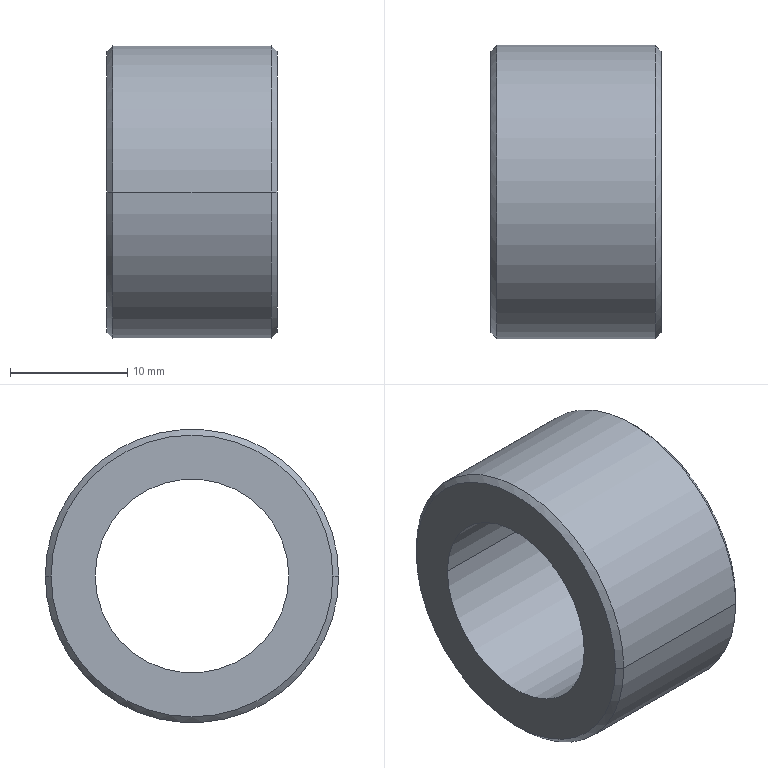Part | STEP file | J452-EBZ05-06-04 | 1 solid | 10 faces | box 14.5 x 25 x 25 mm | volume 3998 mm3 | cone 4 | cylinder 4 | plane 2 | commonest cylinder face diameters 16.5 x2 25 x2
STEP:
#1=CARTESIAN_POINT('',(0.,0.,0.));
#2=DIRECTION('',(0.,0.,1.));
#3=DIRECTION('',(1.,0.,0.));
#4=AXIS2_PLACEMENT_3D('',#1,#2,#3);
#5=CARTESIAN_POINT('',(14.5,-12.,0.));
#6=VERTEX_POINT('',#5);
#7=CARTESIAN_POINT('',(14.5,12.,0.));
#8=VERTEX_POINT('',#7);
#9=CARTESIAN_POINT('',(14.5,0.,0.));
#10=DIRECTION('',(1.,0.,0.));
#11=DIRECTION('',(0.,-1.,0.));
#12=AXIS2_PLACEMENT_3D('',#9,#10,#11);
#13=CIRCLE('',#12,12.);
#14=CARTESIAN_POINT('',(14.,0.,0.));
#15=DIRECTION('',(-1.,0.,0.));
#16=DIRECTION('',(0.,1.,0.));
#17=AXIS2_PLACEMENT_3D('',#14,#15,#16);
#18=CONICAL_SURFACE('',#17,12.5,0.7854);
#19=CARTESIAN_POINT('',(3.142,-0.5));
#20=DIRECTION('',(-1.,0.));
#21=VECTOR('',#20,1.);
#22=LINE('',#19,#21);
#23=(GEOMETRIC_REPRESENTATION_CONTEXT(2)PARAMETRIC_REPRESENTATION_CONTEXT()REPRESENTATION_CONTEXT('',''));
#24=DEFINITIONAL_REPRESENTATION('',(#22),#23);
#25=PCURVE('',#18,#24);
#26=CARTESIAN_POINT('',(14.5,0.,0.));
#27=DIRECTION('',(1.,0.,0.));
#28=DIRECTION('',(0.,-1.,0.));
#29=AXIS2_PLACEMENT_3D('',#26,#27,#28);
#30=PLANE('',#29);
#31=CARTESIAN_POINT('',(0.,0.));
#32=DIRECTION('',(1.,0.));
#33=AXIS2_PLACEMENT_2D('',#31,#32);
#34=CIRCLE('',#33,12.);
#35=(GEOMETRIC_REPRESENTATION_CONTEXT(2)PARAMETRIC_REPRESENTATION_CONTEXT()REPRESENTATION_CONTEXT('',''));
#36=DEFINITIONAL_REPRESENTATION('',(#34),#35);
#37=PCURVE('',#30,#36);
#38=SURFACE_CURVE('',#13,(#25,#37),.PCURVE_S1.);
#39=EDGE_CURVE('',#6,#8,#38,.T.);
#40=ORIENTED_EDGE('',*,*,#39,.F.);
#41=CARTESIAN_POINT('',(14.,-12.5,0.));
#42=VERTEX_POINT('',#41);
#43=CARTESIAN_POINT('',(14.,-12.5,0.));
#44=DIRECTION('',(-0.7071,-0.7071,0.));
#45=VECTOR('',#44,1.);
#46=LINE('',#43,#45);
#47=CARTESIAN_POINT('',(3.142,0.));
#48=DIRECTION('',(0.,1.));
#49=VECTOR('',#48,1.);
#50=LINE('',#47,#49);
#51=(GEOMETRIC_REPRESENTATION_CONTEXT(2)PARAMETRIC_REPRESENTATION_CONTEXT()REPRESENTATION_CONTEXT('',''));
#52=DEFINITIONAL_REPRESENTATION('',(#50),#51);
#53=PCURVE('',#18,#52);
#54=CARTESIAN_POINT('',(14.,0.,0.));
#55=DIRECTION('',(-1.,0.,0.));
#56=DIRECTION('',(0.,1.,0.));
#57=AXIS2_PLACEMENT_3D('',#54,#55,#56);
#58=CONICAL_SURFACE('',#57,12.5,0.7854);
#59=CARTESIAN_POINT('',(3.142,0.));
#60=DIRECTION('',(0.,1.));
#61=VECTOR('',#60,1.);
#62=LINE('',#59,#61);
#63=(GEOMETRIC_REPRESENTATION_CONTEXT(2)PARAMETRIC_REPRESENTATION_CONTEXT()REPRESENTATION_CONTEXT('',''));
#64=DEFINITIONAL_REPRESENTATION('',(#62),#63);
#65=PCURVE('',#58,#64);
#66=SURFACE_CURVE('',#46,(#53,#65),.PCURVE_S1.);
#67=EDGE_CURVE('',#6,#42,#66,.T.);
#68=ORIENTED_EDGE('',*,*,#67,.T.);
#69=CARTESIAN_POINT('',(14.,12.5,0.));
#70=VERTEX_POINT('',#69);
#71=CARTESIAN_POINT('',(14.,0.,0.));
#72=DIRECTION('',(-1.,0.,0.));
#73=DIRECTION('',(0.,-1.,0.));
#74=AXIS2_PLACEMENT_3D('',#71,#72,#73);
#75=CIRCLE('',#74,12.5);
#76=CARTESIAN_POINT('',(-3.142,0.));
#77=DIRECTION('',(1.,0.));
#78=VECTOR('',#77,1.);
#79=LINE('',#76,#78);
#80=(GEOMETRIC_REPRESENTATION_CONTEXT(2)PARAMETRIC_REPRESENTATION_CONTEXT()REPRESENTATION_CONTEXT('',''));
#81=DEFINITIONAL_REPRESENTATION('',(#79),#80);
#82=PCURVE('',#18,#81);
#83=CARTESIAN_POINT('',(0.,0.,0.));
#84=DIRECTION('',(1.,0.,0.));
#85=DIRECTION('',(0.,-1.,0.));
#86=AXIS2_PLACEMENT_3D('',#83,#84,#85);
#87=CYLINDRICAL_SURFACE('',#86,12.5);
#88=CARTESIAN_POINT('',(6.283,14.));
#89=DIRECTION('',(-1.,0.));
#90=VECTOR('',#89,1.);
#91=LINE('',#88,#90);
#92=(GEOMETRIC_REPRESENTATION_CONTEXT(2)PARAMETRIC_REPRESENTATION_CONTEXT()REPRESENTATION_CONTEXT('',''));
#93=DEFINITIONAL_REPRESENTATION('',(#91),#92);
#94=PCURVE('',#87,#93);
#95=SURFACE_CURVE('',#75,(#82,#94),.PCURVE_S1.);
#96=EDGE_CURVE('',#70,#42,#95,.T.);
#97=ORIENTED_EDGE('',*,*,#96,.F.);
#98=CARTESIAN_POINT('',(14.,12.5,0.));
#99=DIRECTION('',(-0.7071,0.7071,0.));
#100=VECTOR('',#99,1.);
#101=LINE('',#98,#100);
#102=CARTESIAN_POINT('',(0.,0.));
#103=DIRECTION('',(0.,1.));
#104=VECTOR('',#103,1.);
#105=LINE('',#102,#104);
#106=(GEOMETRIC_REPRESENTATION_CONTEXT(2)PARAMETRIC_REPRESENTATION_CONTEXT()REPRESENTATION_CONTEXT('',''));
#107=DEFINITIONAL_REPRESENTATION('',(#105),#106);
#108=PCURVE('',#18,#107);
#109=CARTESIAN_POINT('',(6.283,0.));
#110=DIRECTION('',(0.,1.));
#111=VECTOR('',#110,1.);
#112=LINE('',#109,#111);
#113=(GEOMETRIC_REPRESENTATION_CONTEXT(2)PARAMETRIC_REPRESENTATION_CONTEXT()REPRESENTATION_CONTEXT('',''));
#114=DEFINITIONAL_REPRESENTATION('',(#112),#113);
#115=PCURVE('',#58,#114);
#116=SURFACE_CURVE('',#101,(#108,#115),.PCURVE_S1.);
#117=EDGE_CURVE('',#8,#70,#116,.T.);
#118=ORIENTED_EDGE('',*,*,#117,.F.);
#119=EDGE_LOOP('',(#40,#68,#97,#118));
#120=FACE_BOUND('',#119,.T.);
#121=ADVANCED_FACE('',(#120),#18,.T.);
#122=CARTESIAN_POINT('',(0.,12.,0.));
#123=VERTEX_POINT('',#122);
#124=CARTESIAN_POINT('',(0.,-12.,0.));
#125=VERTEX_POINT('',#124);
#126=CARTESIAN_POINT('',(0.,0.,0.));
#127=DIRECTION('',(-1.,0.,0.));
#128=DIRECTION('',(0.,1.,0.));
#129=AXIS2_PLACEMENT_3D('',#126,#127,#128);
#130=CIRCLE('',#129,12.);
#131=CARTESIAN_POINT('',(0.5,0.,0.));
#132=DIRECTION('',(1.,0.,0.));
#133=DIRECTION('',(0.,-1.,0.));
#134=AXIS2_PLACEMENT_3D('',#131,#132,#133);
#135=CONICAL_SURFACE('',#134,12.5,0.7854);
#136=CARTESIAN_POINT('',(3.142,-0.5));
#137=DIRECTION('',(-1.,0.));
#138=VECTOR('',#137,1.);
#139=LINE('',#136,#138);
#140=(GEOMETRIC_REPRESENTATION_CONTEXT(2)PARAMETRIC_REPRESENTATION_CONTEXT()REPRESENTATION_CONTEXT('',''));
#141=DEFINITIONAL_REPRESENTATION('',(#139),#140);
#142=PCURVE('',#135,#141);
#143=CARTESIAN_POINT('',(0.,0.,0.));
#144=DIRECTION('',(-1.,0.,0.));
#145=DIRECTION('',(0.,1.,0.));
#146=AXIS2_PLACEMENT_3D('',#143,#144,#145);
#147=PLANE('',#146);
#148=CARTESIAN_POINT('',(0.,0.));
#149=DIRECTION('',(1.,0.));
#150=AXIS2_PLACEMENT_2D('',#148,#149);
#151=CIRCLE('',#150,12.);
#152=(GEOMETRIC_REPRESENTATION_CONTEXT(2)PARAMETRIC_REPRESENTATION_CONTEXT()REPRESENTATION_CONTEXT('',''));
#153=DEFINITIONAL_REPRESENTATION('',(#151),#152);
#154=PCURVE('',#147,#153);
#155=SURFACE_CURVE('',#130,(#142,#154),.PCURVE_S1.);
#156=EDGE_CURVE('',#123,#125,#155,.T.);
#157=ORIENTED_EDGE('',*,*,#156,.F.);
#158=CARTESIAN_POINT('',(0.5,12.5,0.));
#159=VERTEX_POINT('',#158);
#160=CARTESIAN_POINT('',(0.5,12.5,0.));
#161=DIRECTION('',(0.7071,0.7071,0.));
#162=VECTOR('',#161,1.);
#163=LINE('',#160,#162);
#164=CARTESIAN_POINT('',(3.142,0.));
#165=DIRECTION('',(0.,1.));
#166=VECTOR('',#165,1.);
#167=LINE('',#164,#166);
#168=(GEOMETRIC_REPRESENTATION_CONTEXT(2)PARAMETRIC_REPRESENTATION_CONTEXT()REPRESENTATION_CONTEXT('',''));
#169=DEFINITIONAL_REPRESENTATION('',(#167),#168);
#170=PCURVE('',#135,#169);
#171=CARTESIAN_POINT('',(0.5,0.,0.));
#172=DIRECTION('',(1.,0.,0.));
#173=DIRECTION('',(0.,-1.,0.));
#174=AXIS2_PLACEMENT_3D('',#171,#172,#173);
#175=CONICAL_SURFACE('',#174,12.5,0.7854);
#176=CARTESIAN_POINT('',(3.142,0.));
#177=DIRECTION('',(0.,1.));
#178=VECTOR('',#177,1.);
#179=LINE('',#176,#178);
#180=(GEOMETRIC_REPRESENTATION_CONTEXT(2)PARAMETRIC_REPRESENTATION_CONTEXT()REPRESENTATION_CONTEXT('',''));
#181=DEFINITIONAL_REPRESENTATION('',(#179),#180);
#182=PCURVE('',#175,#181);
#183=SURFACE_CURVE('',#163,(#170,#182),.PCURVE_S1.);
#184=EDGE_CURVE('',#123,#159,#183,.T.);
#185=ORIENTED_EDGE('',*,*,#184,.T.);
#186=CARTESIAN_POINT('',(0.5,-12.5,0.));
#187=VERTEX_POINT('',#186);
#188=CARTESIAN_POINT('',(0.5,0.,0.));
#189=DIRECTION('',(1.,0.,0.));
#190=DIRECTION('',(0.,1.,0.));
#191=AXIS2_PLACEMENT_3D('',#188,#189,#190);
#192=CIRCLE('',#191,12.5);
#193=CARTESIAN_POINT('',(-3.142,0.));
#194=DIRECTION('',(1.,0.));
#195=VECTOR('',#194,1.);
#196=LINE('',#193,#195);
#197=(GEOMETRIC_REPRESENTATION_CONTEXT(2)PARAMETRIC_REPRESENTATION_CONTEXT()REPRESENTATION_CONTEXT('',''));
#198=DEFINITIONAL_REPRESENTATION('',(#196),#197);
#199=PCURVE('',#135,#198);
#200=CARTESIAN_POINT('',(-3.142,0.5));
#201=DIRECTION('',(1.,0.));
#202=VECTOR('',#201,1.);
#203=LINE('',#200,#202);
#204=(GEOMETRIC_REPRESENTATION_CONTEXT(2)PARAMETRIC_REPRESENTATION_CONTEXT()REPRESENTATION_CONTEXT('',''));
#205=DEFINITIONAL_REPRESENTATION('',(#203),#204);
#206=PCURVE('',#87,#205);
#207=SURFACE_CURVE('',#192,(#199,#206),.PCURVE_S1.);
#208=EDGE_CURVE('',#187,#159,#207,.T.);
#209=ORIENTED_EDGE('',*,*,#208,.F.);
#210=CARTESIAN_POINT('',(0.5,-12.5,0.));
#211=DIRECTION('',(0.7071,-0.7071,0.));
#212=VECTOR('',#211,1.);
#213=LINE('',#210,#212);
#214=CARTESIAN_POINT('',(0.,0.));
#215=DIRECTION('',(0.,1.));
#216=VECTOR('',#215,1.);
#217=LINE('',#214,#216);
#218=(GEOMETRIC_REPRESENTATION_CONTEXT(2)PARAMETRIC_REPRESENTATION_CONTEXT()REPRESENTATION_CONTEXT('',''));
#219=DEFINITIONAL_REPRESENTATION('',(#217),#218);
#220=PCURVE('',#135,#219);
#221=CARTESIAN_POINT('',(6.283,0.));
#222=DIRECTION('',(0.,1.));
#223=VECTOR('',#222,1.);
#224=LINE('',#221,#223);
#225=(GEOMETRIC_REPRESENTATION_CONTEXT(2)PARAMETRIC_REPRESENTATION_CONTEXT()REPRESENTATION_CONTEXT('',''));
#226=DEFINITIONAL_REPRESENTATION('',(#224),#225);
#227=PCURVE('',#175,#226);
#228=SURFACE_CURVE('',#213,(#220,#227),.PCURVE_S1.);
#229=EDGE_CURVE('',#125,#187,#228,.T.);
#230=ORIENTED_EDGE('',*,*,#229,.F.);
#231=EDGE_LOOP('',(#157,#185,#209,#230));
#232=FACE_BOUND('',#231,.T.);
#233=ADVANCED_FACE('',(#232),#135,.T.);
#234=CARTESIAN_POINT('',(14.5,8.25,0.));
#235=VERTEX_POINT('',#234);
#236=CARTESIAN_POINT('',(0.,8.25,0.));
#237=VERTEX_POINT('',#236);
#238=CARTESIAN_POINT('',(14.5,8.25,0.));
#239=DIRECTION('',(-1.,0.,0.));
#240=VECTOR('',#239,1.);
#241=LINE('',#238,#240);
#242=CARTESIAN_POINT('',(14.5,0.,0.));
#243=DIRECTION('',(-1.,0.,0.));
#244=DIRECTION('',(0.,1.,0.));
#245=AXIS2_PLACEMENT_3D('',#242,#243,#244);
#246=CYLINDRICAL_SURFACE('',#245,8.25);
#247=CARTESIAN_POINT('',(6.283,0.));
#248=DIRECTION('',(0.,1.));
#249=VECTOR('',#248,1.);
#250=LINE('',#247,#249);
#251=(GEOMETRIC_REPRESENTATION_CONTEXT(2)PARAMETRIC_REPRESENTATION_CONTEXT()REPRESENTATION_CONTEXT('',''));
#252=DEFINITIONAL_REPRESENTATION('',(#250),#251);
#253=PCURVE('',#246,#252);
#254=CARTESIAN_POINT('',(14.5,0.,0.));
#255=DIRECTION('',(-1.,0.,0.));
#256=DIRECTION('',(0.,1.,0.));
#257=AXIS2_PLACEMENT_3D('',#254,#255,#256);
#258=CYLINDRICAL_SURFACE('',#257,8.25);
#259=CARTESIAN_POINT('',(0.,0.));
#260=DIRECTION('',(0.,1.));
#261=VECTOR('',#260,1.);
#262=LINE('',#259,#261);
#263=(GEOMETRIC_REPRESENTATION_CONTEXT(2)PARAMETRIC_REPRESENTATION_CONTEXT()REPRESENTATION_CONTEXT('',''));
#264=DEFINITIONAL_REPRESENTATION('',(#262),#263);
#265=PCURVE('',#258,#264);
#266=SURFACE_CURVE('',#241,(#253,#265),.PCURVE_S1.);
#267=EDGE_CURVE('',#235,#237,#266,.T.);
#268=ORIENTED_EDGE('',*,*,#267,.T.);
#269=CARTESIAN_POINT('',(0.,-8.25,0.));
#270=VERTEX_POINT('',#269);
#271=CARTESIAN_POINT('',(0.,0.,0.));
#272=DIRECTION('',(1.,0.,0.));
#273=DIRECTION('',(0.,-1.,0.));
#274=AXIS2_PLACEMENT_3D('',#271,#272,#273);
#275=CIRCLE('',#274,8.25);
#276=CARTESIAN_POINT('',(9.425,14.5));
#277=DIRECTION('',(-1.,0.));
#278=VECTOR('',#277,1.);
#279=LINE('',#276,#278);
#280=(GEOMETRIC_REPRESENTATION_CONTEXT(2)PARAMETRIC_REPRESENTATION_CONTEXT()REPRESENTATION_CONTEXT('',''));
#281=DEFINITIONAL_REPRESENTATION('',(#279),#280);
#282=PCURVE('',#246,#281);
#283=CARTESIAN_POINT('',(-8.25,0.));
#284=CARTESIAN_POINT('',(-8.25,14.289));
#285=CARTESIAN_POINT('',(4.125,7.145));
#286=CARTESIAN_POINT('',(16.5,0.));
#287=CARTESIAN_POINT('',(4.125,-7.145));
#288=CARTESIAN_POINT('',(-8.25,-14.289));
#289=CARTESIAN_POINT('',(-8.25,0.));
#290=(BOUNDED_CURVE()B_SPLINE_CURVE(2,(#283,#284,#285,#286,#287,#288,#289),.UNSPECIFIED.,.T.,.F.)B_SPLINE_CURVE_WITH_KNOTS((1,2,2,2,2,1),(-2.094,0.,2.094,4.189,6.283,8.378),.UNSPECIFIED.)CURVE()GEOMETRIC_REPRESENTATION_ITEM()RATIONAL_B_SPLINE_CURVE((1.,0.5,1.,0.5,1.,0.5,1.))REPRESENTATION_ITEM(''));
#291=(GEOMETRIC_REPRESENTATION_CONTEXT(2)PARAMETRIC_REPRESENTATION_CONTEXT()REPRESENTATION_CONTEXT('',''));
#292=DEFINITIONAL_REPRESENTATION('',(#290),#291);
#293=PCURVE('',#147,#292);
#294=SURFACE_CURVE('',#275,(#282,#293),.PCURVE_S1.);
#295=EDGE_CURVE('',#237,#270,#294,.T.);
#296=ORIENTED_EDGE('',*,*,#295,.T.);
#297=CARTESIAN_POINT('',(14.5,-8.25,0.));
#298=VERTEX_POINT('',#297);
#299=CARTESIAN_POINT('',(14.5,-8.25,0.));
#300=DIRECTION('',(-1.,0.,0.));
#301=VECTOR('',#300,1.);
#302=LINE('',#299,#301);
#303=CARTESIAN_POINT('',(3.142,0.));
#304=DIRECTION('',(0.,1.));
#305=VECTOR('',#304,1.);
#306=LINE('',#303,#305);
#307=(GEOMETRIC_REPRESENTATION_CONTEXT(2)PARAMETRIC_REPRESENTATION_CONTEXT()REPRESENTATION_CONTEXT('',''));
#308=DEFINITIONAL_REPRESENTATION('',(#306),#307);
#309=PCURVE('',#246,#308);
#310=CARTESIAN_POINT('',(3.142,0.));
#311=DIRECTION('',(0.,1.));
#312=VECTOR('',#311,1.);
#313=LINE('',#310,#312);
#314=(GEOMETRIC_REPRESENTATION_CONTEXT(2)PARAMETRIC_REPRESENTATION_CONTEXT()REPRESENTATION_CONTEXT('',''));
#315=DEFINITIONAL_REPRESENTATION('',(#313),#314);
#316=PCURVE('',#258,#315);
#317=SURFACE_CURVE('',#302,(#309,#316),.PCURVE_S1.);
#318=EDGE_CURVE('',#298,#270,#317,.T.);
#319=ORIENTED_EDGE('',*,*,#318,.F.);
#320=CARTESIAN_POINT('',(14.5,0.,0.));
#321=DIRECTION('',(-1.,0.,0.));
#322=DIRECTION('',(0.,1.,0.));
#323=AXIS2_PLACEMENT_3D('',#320,#321,#322);
#324=CIRCLE('',#323,8.25);
#325=CARTESIAN_POINT('',(0.,0.));
#326=DIRECTION('',(1.,0.));
#327=VECTOR('',#326,1.);
#328=LINE('',#325,#327);
#329=(GEOMETRIC_REPRESENTATION_CONTEXT(2)PARAMETRIC_REPRESENTATION_CONTEXT()REPRESENTATION_CONTEXT('',''));
#330=DEFINITIONAL_REPRESENTATION('',(#328),#329);
#331=PCURVE('',#246,#330);
#332=CARTESIAN_POINT('',(-8.25,0.));
#333=CARTESIAN_POINT('',(-8.25,14.289));
#334=CARTESIAN_POINT('',(4.125,7.145));
#335=CARTESIAN_POINT('',(16.5,0.));
#336=CARTESIAN_POINT('',(4.125,-7.145));
#337=CARTESIAN_POINT('',(-8.25,-14.289));
#338=CARTESIAN_POINT('',(-8.25,0.));
#339=(BOUNDED_CURVE()B_SPLINE_CURVE(2,(#332,#333,#334,#335,#336,#337,#338),.UNSPECIFIED.,.T.,.F.)B_SPLINE_CURVE_WITH_KNOTS((1,2,2,2,2,1),(-2.094,0.,2.094,4.189,6.283,8.378),.UNSPECIFIED.)CURVE()GEOMETRIC_REPRESENTATION_ITEM()RATIONAL_B_SPLINE_CURVE((1.,0.5,1.,0.5,1.,0.5,1.))REPRESENTATION_ITEM(''));
#340=(GEOMETRIC_REPRESENTATION_CONTEXT(2)PARAMETRIC_REPRESENTATION_CONTEXT()REPRESENTATION_CONTEXT('',''));
#341=DEFINITIONAL_REPRESENTATION('',(#339),#340);
#342=PCURVE('',#30,#341);
#343=SURFACE_CURVE('',#324,(#331,#342),.PCURVE_S1.);
#344=EDGE_CURVE('',#298,#235,#343,.T.);
#345=ORIENTED_EDGE('',*,*,#344,.T.);
#346=EDGE_LOOP('',(#268,#296,#319,#345));
#347=FACE_BOUND('',#346,.F.);
#348=ADVANCED_FACE('',(#347),#246,.F.);
#349=ORIENTED_EDGE('',*,*,#208,.T.);
#350=CARTESIAN_POINT('',(0.,12.5,0.));
#351=DIRECTION('',(1.,0.,0.));
#352=VECTOR('',#351,1.);
#353=LINE('',#350,#352);
#354=CARTESIAN_POINT('',(3.142,0.));
#355=DIRECTION('',(0.,1.));
#356=VECTOR('',#355,1.);
#357=LINE('',#354,#356);
#358=(GEOMETRIC_REPRESENTATION_CONTEXT(2)PARAMETRIC_REPRESENTATION_CONTEXT()REPRESENTATION_CONTEXT('',''));
#359=DEFINITIONAL_REPRESENTATION('',(#357),#358);
#360=PCURVE('',#87,#359);
#361=CARTESIAN_POINT('',(0.,0.,0.));
#362=DIRECTION('',(1.,0.,0.));
#363=DIRECTION('',(0.,-1.,0.));
#364=AXIS2_PLACEMENT_3D('',#361,#362,#363);
#365=CYLINDRICAL_SURFACE('',#364,12.5);
#366=CARTESIAN_POINT('',(3.142,0.));
#367=DIRECTION('',(0.,1.));
#368=VECTOR('',#367,1.);
#369=LINE('',#366,#368);
#370=(GEOMETRIC_REPRESENTATION_CONTEXT(2)PARAMETRIC_REPRESENTATION_CONTEXT()REPRESENTATION_CONTEXT('',''));
#371=DEFINITIONAL_REPRESENTATION('',(#369),#370);
#372=PCURVE('',#365,#371);
#373=SURFACE_CURVE('',#353,(#360,#372),.PCURVE_S1.);
#374=EDGE_CURVE('',#159,#70,#373,.T.);
#375=ORIENTED_EDGE('',*,*,#374,.T.);
#376=ORIENTED_EDGE('',*,*,#96,.T.);
#377=CARTESIAN_POINT('',(0.,-12.5,0.));
#378=DIRECTION('',(1.,0.,0.));
#379=VECTOR('',#378,1.);
#380=LINE('',#377,#379);
#381=CARTESIAN_POINT('',(0.,0.));
#382=DIRECTION('',(0.,1.));
#383=VECTOR('',#382,1.);
#384=LINE('',#381,#383);
#385=(GEOMETRIC_REPRESENTATION_CONTEXT(2)PARAMETRIC_REPRESENTATION_CONTEXT()REPRESENTATION_CONTEXT('',''));
#386=DEFINITIONAL_REPRESENTATION('',(#384),#385);
#387=PCURVE('',#87,#386);
#388=CARTESIAN_POINT('',(6.283,0.));
#389=DIRECTION('',(0.,1.));
#390=VECTOR('',#389,1.);
#391=LINE('',#388,#390);
#392=(GEOMETRIC_REPRESENTATION_CONTEXT(2)PARAMETRIC_REPRESENTATION_CONTEXT()REPRESENTATION_CONTEXT('',''));
#393=DEFINITIONAL_REPRESENTATION('',(#391),#392);
#394=PCURVE('',#365,#393);
#395=SURFACE_CURVE('',#380,(#387,#394),.PCURVE_S1.);
#396=EDGE_CURVE('',#187,#42,#395,.T.);
#397=ORIENTED_EDGE('',*,*,#396,.F.);
#398=EDGE_LOOP('',(#349,#375,#376,#397));
#399=FACE_BOUND('',#398,.T.);
#400=ADVANCED_FACE('',(#399),#87,.T.);
#401=CARTESIAN_POINT('',(14.5,0.,0.));
#402=DIRECTION('',(1.,0.,0.));
#403=DIRECTION('',(0.,-1.,0.));
#404=AXIS2_PLACEMENT_3D('',#401,#402,#403);
#405=CIRCLE('',#404,12.);
#406=CARTESIAN_POINT('',(0.,0.));
#407=DIRECTION('',(1.,0.));
#408=AXIS2_PLACEMENT_2D('',#406,#407);
#409=CIRCLE('',#408,12.);
#410=(GEOMETRIC_REPRESENTATION_CONTEXT(2)PARAMETRIC_REPRESENTATION_CONTEXT()REPRESENTATION_CONTEXT('',''));
#411=DEFINITIONAL_REPRESENTATION('',(#409),#410);
#412=PCURVE('',#30,#411);
#413=CARTESIAN_POINT('',(9.425,-0.5));
#414=DIRECTION('',(-1.,0.));
#415=VECTOR('',#414,1.);
#416=LINE('',#413,#415);
#417=(GEOMETRIC_REPRESENTATION_CONTEXT(2)PARAMETRIC_REPRESENTATION_CONTEXT()REPRESENTATION_CONTEXT('',''));
#418=DEFINITIONAL_REPRESENTATION('',(#416),#417);
#419=PCURVE('',#58,#418);
#420=SURFACE_CURVE('',#405,(#412,#419),.PCURVE_S1.);
#421=EDGE_CURVE('',#8,#6,#420,.T.);
#422=ORIENTED_EDGE('',*,*,#421,.T.);
#423=ORIENTED_EDGE('',*,*,#39,.T.);
#424=EDGE_LOOP('',(#422,#423));
#425=FACE_BOUND('',#424,.T.);
#426=CARTESIAN_POINT('',(14.5,0.,0.));
#427=DIRECTION('',(-1.,0.,0.));
#428=DIRECTION('',(0.,1.,0.));
#429=AXIS2_PLACEMENT_3D('',#426,#427,#428);
#430=CIRCLE('',#429,8.25);
#431=CARTESIAN_POINT('',(-8.25,0.));
#432=CARTESIAN_POINT('',(-8.25,14.289));
#433=CARTESIAN_POINT('',(4.125,7.145));
#434=CARTESIAN_POINT('',(16.5,0.));
#435=CARTESIAN_POINT('',(4.125,-7.145));
#436=CARTESIAN_POINT('',(-8.25,-14.289));
#437=CARTESIAN_POINT('',(-8.25,0.));
#438=(BOUNDED_CURVE()B_SPLINE_CURVE(2,(#431,#432,#433,#434,#435,#436,#437),.UNSPECIFIED.,.T.,.F.)B_SPLINE_CURVE_WITH_KNOTS((1,2,2,2,2,1),(-2.094,0.,2.094,4.189,6.283,8.378),.UNSPECIFIED.)CURVE()GEOMETRIC_REPRESENTATION_ITEM()RATIONAL_B_SPLINE_CURVE((1.,0.5,1.,0.5,1.,0.5,1.))REPRESENTATION_ITEM(''));
#439=(GEOMETRIC_REPRESENTATION_CONTEXT(2)PARAMETRIC_REPRESENTATION_CONTEXT()REPRESENTATION_CONTEXT('',''));
#440=DEFINITIONAL_REPRESENTATION('',(#438),#439);
#441=PCURVE('',#30,#440);
#442=CARTESIAN_POINT('',(0.,0.));
#443=DIRECTION('',(1.,0.));
#444=VECTOR('',#443,1.);
#445=LINE('',#442,#444);
#446=(GEOMETRIC_REPRESENTATION_CONTEXT(2)PARAMETRIC_REPRESENTATION_CONTEXT()REPRESENTATION_CONTEXT('',''));
#447=DEFINITIONAL_REPRESENTATION('',(#445),#446);
#448=PCURVE('',#258,#447);
#449=SURFACE_CURVE('',#430,(#441,#448),.PCURVE_S1.);
#450=EDGE_CURVE('',#235,#298,#449,.T.);
#451=ORIENTED_EDGE('',*,*,#450,.T.);
#452=ORIENTED_EDGE('',*,*,#344,.T.);
#453=EDGE_LOOP('',(#451,#452));
#454=FACE_BOUND('',#453,.T.);
#455=ADVANCED_FACE('',(#425,#454),#30,.T.);
#456=CARTESIAN_POINT('',(0.,0.,0.));
#457=DIRECTION('',(-1.,0.,0.));
#458=DIRECTION('',(0.,1.,0.));
#459=AXIS2_PLACEMENT_3D('',#456,#457,#458);
#460=CIRCLE('',#459,12.);
#461=CARTESIAN_POINT('',(0.,0.));
#462=DIRECTION('',(1.,0.));
#463=AXIS2_PLACEMENT_2D('',#461,#462);
#464=CIRCLE('',#463,12.);
#465=(GEOMETRIC_REPRESENTATION_CONTEXT(2)PARAMETRIC_REPRESENTATION_CONTEXT()REPRESENTATION_CONTEXT('',''));
#466=DEFINITIONAL_REPRESENTATION('',(#464),#465);
#467=PCURVE('',#147,#466);
#468=CARTESIAN_POINT('',(9.425,-0.5));
#469=DIRECTION('',(-1.,0.));
#470=VECTOR('',#469,1.);
#471=LINE('',#468,#470);
#472=(GEOMETRIC_REPRESENTATION_CONTEXT(2)PARAMETRIC_REPRESENTATION_CONTEXT()REPRESENTATION_CONTEXT('',''));
#473=DEFINITIONAL_REPRESENTATION('',(#471),#472);
#474=PCURVE('',#175,#473);
#475=SURFACE_CURVE('',#460,(#467,#474),.PCURVE_S1.);
#476=EDGE_CURVE('',#125,#123,#475,.T.);
#477=ORIENTED_EDGE('',*,*,#476,.T.);
#478=ORIENTED_EDGE('',*,*,#156,.T.);
#479=EDGE_LOOP('',(#477,#478));
#480=FACE_BOUND('',#479,.T.);
#481=ORIENTED_EDGE('',*,*,#295,.T.);
#482=CARTESIAN_POINT('',(0.,0.,0.));
#483=DIRECTION('',(1.,0.,0.));
#484=DIRECTION('',(0.,-1.,0.));
#485=AXIS2_PLACEMENT_3D('',#482,#483,#484);
#486=CIRCLE('',#485,8.25);
#487=CARTESIAN_POINT('',(-8.25,0.));
#488=CARTESIAN_POINT('',(-8.25,14.289));
#489=CARTESIAN_POINT('',(4.125,7.145));
#490=CARTESIAN_POINT('',(16.5,0.));
#491=CARTESIAN_POINT('',(4.125,-7.145));
#492=CARTESIAN_POINT('',(-8.25,-14.289));
#493=CARTESIAN_POINT('',(-8.25,0.));
#494=(BOUNDED_CURVE()B_SPLINE_CURVE(2,(#487,#488,#489,#490,#491,#492,#493),.UNSPECIFIED.,.T.,.F.)B_SPLINE_CURVE_WITH_KNOTS((1,2,2,2,2,1),(-2.094,0.,2.094,4.189,6.283,8.378),.UNSPECIFIED.)CURVE()GEOMETRIC_REPRESENTATION_ITEM()RATIONAL_B_SPLINE_CURVE((1.,0.5,1.,0.5,1.,0.5,1.))REPRESENTATION_ITEM(''));
#495=(GEOMETRIC_REPRESENTATION_CONTEXT(2)PARAMETRIC_REPRESENTATION_CONTEXT()REPRESENTATION_CONTEXT('',''));
#496=DEFINITIONAL_REPRESENTATION('',(#494),#495);
#497=PCURVE('',#147,#496);
#498=CARTESIAN_POINT('',(3.142,14.5));
#499=DIRECTION('',(-1.,0.));
#500=VECTOR('',#499,1.);
#501=LINE('',#498,#500);
#502=(GEOMETRIC_REPRESENTATION_CONTEXT(2)PARAMETRIC_REPRESENTATION_CONTEXT()REPRESENTATION_CONTEXT('',''));
#503=DEFINITIONAL_REPRESENTATION('',(#501),#502);
#504=PCURVE('',#258,#503);
#505=SURFACE_CURVE('',#486,(#497,#504),.PCURVE_S1.);
#506=EDGE_CURVE('',#270,#237,#505,.T.);
#507=ORIENTED_EDGE('',*,*,#506,.T.);
#508=EDGE_LOOP('',(#481,#507));
#509=FACE_BOUND('',#508,.T.);
#510=ADVANCED_FACE('',(#480,#509),#147,.T.);
#511=ORIENTED_EDGE('',*,*,#374,.F.);
#512=CARTESIAN_POINT('',(0.5,0.,0.));
#513=DIRECTION('',(1.,0.,0.));
#514=DIRECTION('',(0.,1.,0.));
#515=AXIS2_PLACEMENT_3D('',#512,#513,#514);
#516=CIRCLE('',#515,12.5);
#517=CARTESIAN_POINT('',(3.142,0.5));
#518=DIRECTION('',(1.,0.));
#519=VECTOR('',#518,1.);
#520=LINE('',#517,#519);
#521=(GEOMETRIC_REPRESENTATION_CONTEXT(2)PARAMETRIC_REPRESENTATION_CONTEXT()REPRESENTATION_CONTEXT('',''));
#522=DEFINITIONAL_REPRESENTATION('',(#520),#521);
#523=PCURVE('',#365,#522);
#524=CARTESIAN_POINT('',(3.142,0.));
#525=DIRECTION('',(1.,0.));
#526=VECTOR('',#525,1.);
#527=LINE('',#524,#526);
#528=(GEOMETRIC_REPRESENTATION_CONTEXT(2)PARAMETRIC_REPRESENTATION_CONTEXT()REPRESENTATION_CONTEXT('',''));
#529=DEFINITIONAL_REPRESENTATION('',(#527),#528);
#530=PCURVE('',#175,#529);
#531=SURFACE_CURVE('',#516,(#523,#530),.PCURVE_S1.);
#532=EDGE_CURVE('',#159,#187,#531,.T.);
#533=ORIENTED_EDGE('',*,*,#532,.T.);
#534=ORIENTED_EDGE('',*,*,#396,.T.);
#535=CARTESIAN_POINT('',(14.,0.,0.));
#536=DIRECTION('',(-1.,0.,0.));
#537=DIRECTION('',(0.,-1.,0.));
#538=AXIS2_PLACEMENT_3D('',#535,#536,#537);
#539=CIRCLE('',#538,12.5);
#540=CARTESIAN_POINT('',(6.283,14.));
#541=DIRECTION('',(-1.,0.));
#542=VECTOR('',#541,1.);
#543=LINE('',#540,#542);
#544=(GEOMETRIC_REPRESENTATION_CONTEXT(2)PARAMETRIC_REPRESENTATION_CONTEXT()REPRESENTATION_CONTEXT('',''));
#545=DEFINITIONAL_REPRESENTATION('',(#543),#544);
#546=PCURVE('',#365,#545);
#547=CARTESIAN_POINT('',(3.142,0.));
#548=DIRECTION('',(1.,0.));
#549=VECTOR('',#548,1.);
#550=LINE('',#547,#549);
#551=(GEOMETRIC_REPRESENTATION_CONTEXT(2)PARAMETRIC_REPRESENTATION_CONTEXT()REPRESENTATION_CONTEXT('',''));
#552=DEFINITIONAL_REPRESENTATION('',(#550),#551);
#553=PCURVE('',#58,#552);
#554=SURFACE_CURVE('',#539,(#546,#553),.PCURVE_S1.);
#555=EDGE_CURVE('',#42,#70,#554,.T.);
#556=ORIENTED_EDGE('',*,*,#555,.T.);
#557=EDGE_LOOP('',(#511,#533,#534,#556));
#558=FACE_BOUND('',#557,.T.);
#559=ADVANCED_FACE('',(#558),#365,.T.);
#560=ORIENTED_EDGE('',*,*,#506,.T.);
#561=ORIENTED_EDGE('',*,*,#267,.F.);
#562=ORIENTED_EDGE('',*,*,#450,.T.);
#563=ORIENTED_EDGE('',*,*,#318,.T.);
#564=EDGE_LOOP('',(#560,#561,#562,#563));
#565=FACE_BOUND('',#564,.F.);
#566=ADVANCED_FACE('',(#565),#258,.F.);
#567=ORIENTED_EDGE('',*,*,#184,.F.);
#568=ORIENTED_EDGE('',*,*,#476,.F.);
#569=ORIENTED_EDGE('',*,*,#229,.T.);
#570=ORIENTED_EDGE('',*,*,#532,.F.);
#571=EDGE_LOOP('',(#567,#568,#569,#570));
#572=FACE_BOUND('',#571,.T.);
#573=ADVANCED_FACE('',(#572),#175,.T.);
#574=ORIENTED_EDGE('',*,*,#67,.F.);
#575=ORIENTED_EDGE('',*,*,#421,.F.);
#576=ORIENTED_EDGE('',*,*,#117,.T.);
#577=ORIENTED_EDGE('',*,*,#555,.F.);
#578=EDGE_LOOP('',(#574,#575,#576,#577));
#579=FACE_BOUND('',#578,.T.);
#580=ADVANCED_FACE('',(#579),#58,.T.);
#581=CLOSED_SHELL('',(#121,#233,#348,#400,#455,#510,#559,#566,#573,#580));
#582=MANIFOLD_SOLID_BREP('',#581);
#583=(LENGTH_UNIT()NAMED_UNIT(*)SI_UNIT(.MILLI.,.METRE.));
#584=UNCERTAINTY_MEASURE_WITH_UNIT(LENGTH_MEASURE(0.0000001),#583,'','');
#585=(NAMED_UNIT(*)PLANE_ANGLE_UNIT()SI_UNIT($,.RADIAN.));
#586=(NAMED_UNIT(*)SI_UNIT($,.STERADIAN.)SOLID_ANGLE_UNIT());
#587=(GEOMETRIC_REPRESENTATION_CONTEXT(3)GLOBAL_UNCERTAINTY_ASSIGNED_CONTEXT((#584))GLOBAL_UNIT_ASSIGNED_CONTEXT((#583,#585,#586))REPRESENTATION_CONTEXT('',''));
#588=ADVANCED_BREP_SHAPE_REPRESENTATION('',(#4,#582),#587);